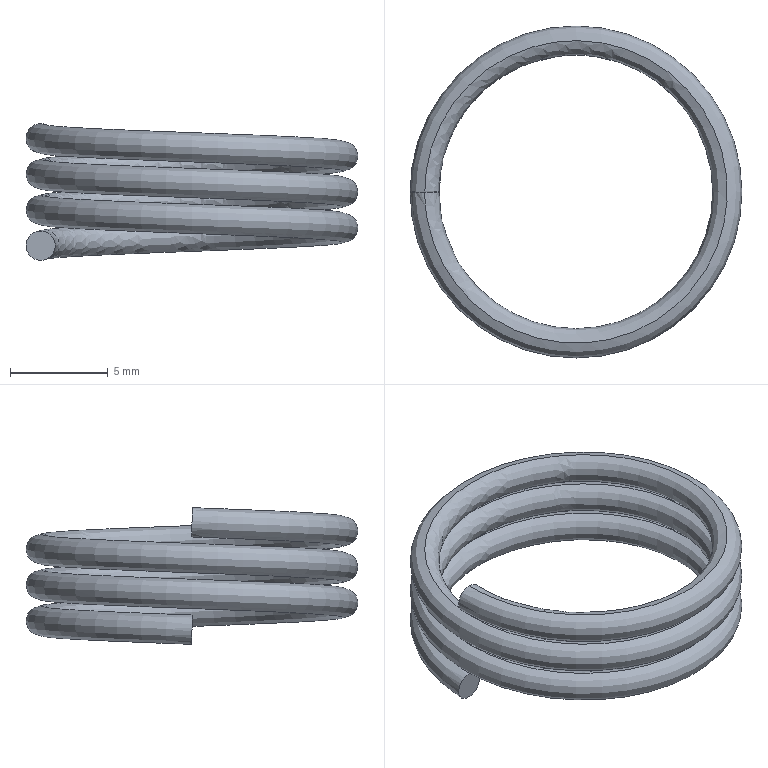Part | SolidWorks | features Helix 1, Sweep 1 | 1 solid | 4 faces | box 17 x 17 x 6.999 mm | volume 258.247 mm3 | spline 2 | plane 2